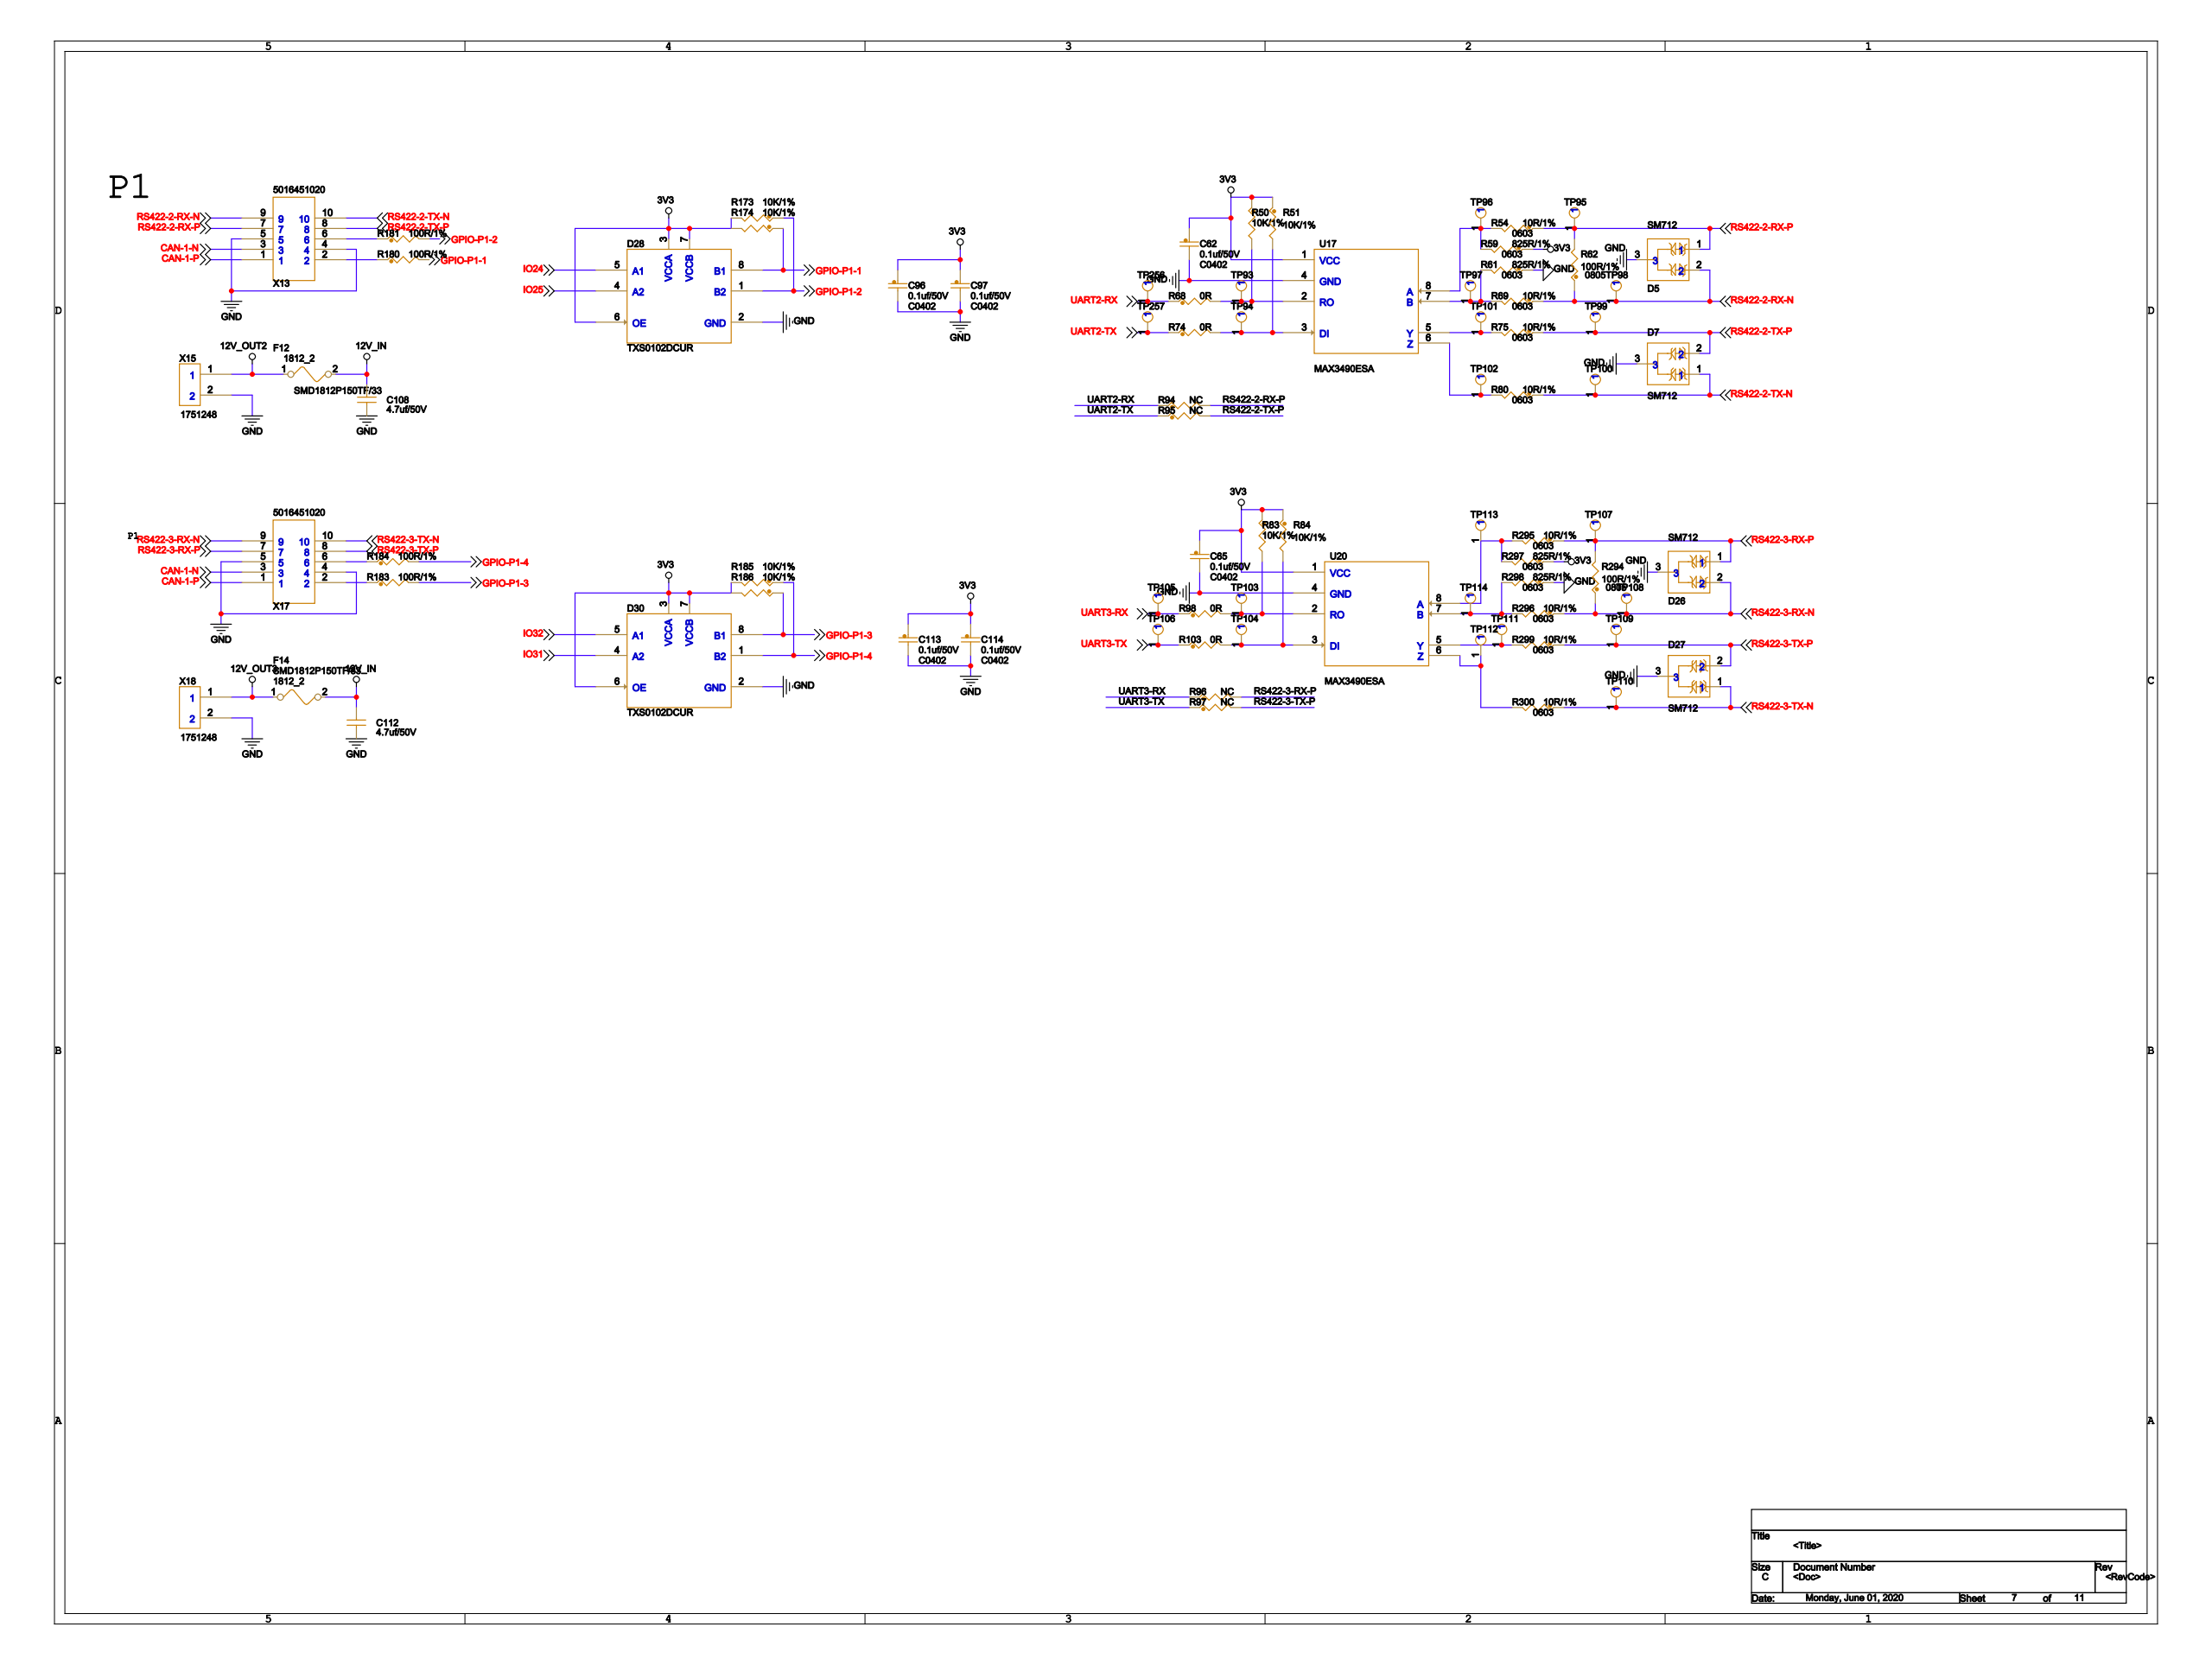Circuit board | Cadence Allegro | 792 parts | 400 nets | one sheet of the schematic
Parts on this sheet (reference | value | footprint):
C62 | 0.1uf/50V | C0402
C65 | 0.1uf/50V | C0402
C96 | 0.1uf/50V | C0402
C97 | 0.1uf/50V | C0402
C108 | 4.7uf/50V | C0805
C112 | 4.7uf/50V | C0805
C113 | 0.1uf/50V | C0402
C114 | 0.1uf/50V | C0402
D5 | SM712 | SOT23
D7 | SM712 | SOT23
D26 | SM712 | SOT23
D27 | SM712 | SOT23
D28 | TXS0102DCUR | VSSOP8
D30 | TXS0102DCUR | VSSOP8
F12 | SMD1812P150TF/33 | 1812_2
F14 | SMD1812P150TF/33 | 1812_2
R50 | 10K/1% | 0402
R51 | 10K/1% | 0402
R54 | 10R/1% | 0603
R59 | 825R/1% | 0603
R61 | 825R/1% | 0603
R62 | 100R/1% | 0805
R68 | 0R | 0603
R69 | 10R/1% | 0603
R74 | 0R | 0603
R75 | 10R/1% | 0603
R80 | 10R/1% | 0603
R83 | 10K/1% | 0402
R84 | 10K/1% | 0402
R94 | NC | 0603
R95 | NC | 0603
R96 | NC | 0603
R97 | NC | 0603
R98 | 0R | 0603
R103 | 0R | 0603
R173 | 10K/1% | 0402
R174 | 10K/1% | 0402
R180 | 100R/1% | 0603
R181 | 100R/1% | 0603
R183 | 100R/1% | 0603
R184 | 100R/1% | 0603
R185 | 10K/1% | 0402
R186 | 10K/1% | 0402
R294 | 100R/1% | 0805
R295 | 10R/1% | 0603
R296 | 10R/1% | 0603
R297 | 825R/1% | 0603
R298 | 825R/1% | 0603
R299 | 10R/1% | 0603
R300 | 10R/1% | 0603
TP93 | TESTPOINT | TESTPOINT-33MIL
TP94 | TESTPOINT | TESTPOINT-33MIL
TP95 | TESTPOINT | TESTPOINT-33MIL
TP96 | TESTPOINT | TESTPOINT-33MIL
TP97 | TESTPOINT | TESTPOINT-33MIL
TP98 | TESTPOINT | TESTPOINT-33MIL
TP99 | TESTPOINT | TESTPOINT-33MIL
TP100 | TESTPOINT | TESTPOINT-33MIL
TP101 | TESTPOINT | TESTPOINT-33MIL
TP102 | TESTPOINT | TESTPOINT-33MIL
TP103 | TESTPOINT | TESTPOINT-33MIL
TP104 | TESTPOINT | TESTPOINT-33MIL
TP105 | TESTPOINT | TESTPOINT-33MIL
TP106 | TESTPOINT | TESTPOINT-33MIL
TP107 | TESTPOINT | TESTPOINT-33MIL
TP108 | TESTPOINT | TESTPOINT-33MIL
TP109 | TESTPOINT | TESTPOINT-33MIL
TP110 | TESTPOINT | TESTPOINT-33MIL
TP111 | TESTPOINT | TESTPOINT-33MIL
TP112 | TESTPOINT | TESTPOINT-33MIL
TP113 | TESTPOINT | TESTPOINT-33MIL
TP114 | TESTPOINT | TESTPOINT-33MIL
TP256 | TESTPOINT | TESTPOINT-33MIL
TP257 | TESTPOINT | TESTPOINT-33MIL
U17 | MAX3490ESA | SOP8
U20 | MAX3490ESA | SOP8
X13 | 5016451020 | 5016451020
X15 | 1751248 | EDG-35-2P
X17 | 5016451020 | 5016451020
X18 | 1751248 | EDG-35-2P
Nets of these parts (net: part-pin ...):
3V3: C62-1 C65-1 C96-1 C97-1 C113-1 C114-1 D28-3 D28-6 D28-7 D30-3 D30-6 D30-7 R50-1 R51-1 R59-1 R83-1 R84-1 R173-2 R174-2 R185-2 R186-2 R297-1 U17-1 U20-1
GND: C62-2 C65-2 C96-2 C97-2 C108-2 C112-2 C113-2 C114-2 D5-3 D7-3 D26-3 D27-3 D28-2 D30-2 R61-1 R298-1 U17-4 U20-4 X13-4 X13-5 X15-2 X17-4 X17-5 X18-2
CAN-1-P: X13-1 X17-1
CAN-1-N: X13-3 X17-3
RS422-2-TX-N: D7-1 R80-1 TP100-1 X13-10
N8038355: R180-1 X13-2
N8038383: R181-1 X13-6
RS422-2-RX-P: D5-1 R54-1 R62-2 R94-2 TP95-1 X13-7
RS422-2-TX-P: D7-2 R75-1 R95-2 TP99-1 X13-8
RS422-2-RX-N: D5-2 R62-1 R69-1 TP98-1 X13-9
RS422-3-TX-N: D27-1 R300-1 TP110-1 X17-10
N8038535: R183-1 X17-2
N8038531: R184-1 X17-6
RS422-3-RX-P: D26-1 R96-2 R294-2 R295-1 TP107-1 X17-7
RS422-3-TX-P: D27-2 R97-2 R299-1 TP109-1 X17-8
RS422-3-RX-N: D26-2 R294-1 R296-1 TP108-1 X17-9
12V_IN: C108-1 C112-1 F12-2 F14-2
UART2-RX: R68-1 R94-1 TP256-1
UART2-TX: R74-1 R95-1 TP257-1
N8045138: R75-2 TP101-1 U17-5
N8044050: R80-2 TP102-1 U17-6
N8044298: R83-2 R98-2 TP103-1 U20-2
N8044306: R84-2 R103-2 TP104-1 U20-3
UART3-RX: R96-1 R98-1 TP105-1
UART3-TX: R97-1 R103-1 TP106-1
N8044862: R299-2 TP111-1 U20-5
N8044458: R300-2 TP112-1 U20-6
N8044322: R295-2 R297-2 TP113-1 U20-8
N8044390: R296-2 R298-2 TP114-1 U20-7
N8044374: R50-2 R68-2 TP93-1 U17-2
N8044382: R51-2 R74-2 TP94-1 U17-3
N8044046: R54-2 R59-2 TP96-1 U17-8
N8045172: R61-2 R69-2 TP97-1 U17-7
12V_OUT2: F12-1 X15-1
12V_OUT3: F14-1 X18-1
IO24: D28-5
IO25: D28-4
GPIO-P1-1: D28-8 R174-1 R180-2
GPIO-P1-2: D28-1 R173-1 R181-2
IO32: D30-5
IO31: D30-4
GPIO-P1-3: D30-8 R183-2 R186-1
GPIO-P1-4: D30-1 R184-2 R185-1